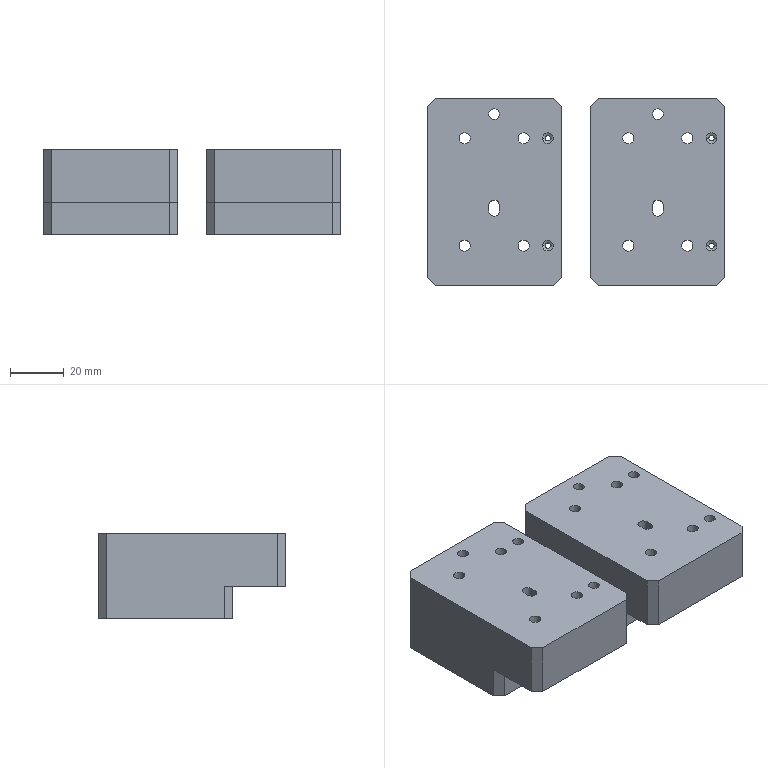NC program | NX | posted with a generic post | part box 111 x 70 x 32 mm
Whole program:
N10 G17 G21 G94 G90
(FLOOR_WALL_COPY , TOOL : D80)
N12 T19 M6
N14 G54
N16 G17 G0 G90 X-43. Y35. S6500 M3
N18 G43 Z30. H19
N20 Z5.
N22 G94 G1 Z2. F1500.
N24 X-40.
N26 X151.
N28 X154.
N30 Z5.
N32 G0 Z30.
N34 X-43.
N36 Z4.
N38 G1 Z1.
N40 X-40.
N42 X151.
N44 X154.
N46 Z4.
N48 G0 Z30.
N50 X-43.
N52 Z3.
N54 G1 Z0.
N56 X-40.
N58 X151.
N60 X154.
N62 Z3.
N64 G0 Z30.
N66 M5
(FLOOR_WALL_1 , TOOL : D10)
N68 T15 M6
N70 G54
N72 G17 G0 G90 X26.443 Y-6.5 S9500 M3
N74 G43 Z30. H15
N76 Z0.508
N78 G94 G1 Z-0.992 F1000.
N80 X25.866 Y-5.5
N82 G3 X25. Y-5. R1.
N84 G1 X0.929 F3500.
N86 X-5. Y0.929
N88 Y20.788
N90 X0.888 Y14.9
N92 X49.112
N94 X55. Y20.788
N96 Y0.929
N98 X49.071 Y-5.
N100 X25.
N102 Y0.
N104 X3.
N106 X0. Y3.
N108 Y9.979
N110 G3 X0.888 Y9.9 R5.
N112 G1 X49.112
N114 G3 X50. Y9.979 R5.
N116 G1 Y3.
N118 X47. Y0.
N120 X25.
N122 Y4.5
N124 X4.864
N126 X4.5 Y4.864
N128 Y5.4
N130 X45.5
N132 Y4.864
N134 X45.136 Y4.5
N136 X25.
N138 G3 X24.134 Y4. R1.
N140 G1 Z0.508
N142 G0 X26.443 Y-6.5 Z-0.483
N144 G1 Z-1.983 F1000.
N146 X25.866 Y-5.5
N148 G3 X25. Y-5. R1.
N150 G1 X0.929 F3500.
N152 X-5. Y0.929
N154 Y20.788
N156 X0.888 Y14.9
N158 X49.112
N160 X55. Y20.788
N162 Y0.929
N164 X49.071 Y-5.
N166 X25.
N168 Y0.
N170 X3.
N172 X0. Y3.
N174 Y9.979
N176 G3 X0.888 Y9.9 R5.
N178 G1 X49.112
N180 G3 X50. Y9.979 R5.
N182 G1 Y3.
N184 X47. Y0.
N186 X25.
N188 Y4.5
N190 X4.864
N192 X4.5 Y4.864
N194 Y5.4
N196 X45.5
N198 Y4.864
N200 X45.136 Y4.5
N202 X25.
N204 G3 X24.134 Y4. R1.
N206 G1 Z-0.483
N208 G0 X26.443 Y-6.5 Z-1.475
N210 G1 Z-2.975 F1000.
N212 X25.866 Y-5.5
N214 G3 X25. Y-5. R1.
N216 G1 X0.929 F3500.
N218 X-5. Y0.929
N220 Y20.788
N222 X0.888 Y14.9
N224 X49.112
N226 X55. Y20.788
N228 Y0.929
N230 X49.071 Y-5.
N232 X25.
N234 Y0.
N236 X3.
N238 X0. Y3.
N240 Y9.979
N242 G3 X0.888 Y9.9 R5.
N244 G1 X49.112
N246 G3 X50. Y9.979 R5.
N248 G1 Y3.
N250 X47. Y0.
N252 X25.
N254 Y4.5
N256 X4.864
N258 X4.5 Y4.864
N260 Y5.4
N262 X45.5
N264 Y4.864
N266 X45.136 Y4.5
N268 X25.
N270 G3 X24.134 Y4. R1.
N272 G1 Z-1.475
N274 G0 X26.443 Y-6.5 Z-2.467
N276 G1 Z-3.967 F1000.
N278 X25.866 Y-5.5
N280 G3 X25. Y-5. R1.
N282 G1 X0.929 F3500.
N284 X-5. Y0.929
N286 Y20.788
N288 X0.888 Y14.9
N290 X49.112
N292 X55. Y20.788
N294 Y0.929
N296 X49.071 Y-5.
N298 X25.
N300 Y0.
N302 X3.
N304 X0. Y3.
N306 Y9.979
N308 G3 X0.888 Y9.9 R5.
N310 G1 X49.112
N312 G3 X50. Y9.979 R5.
N314 G1 Y3.
N316 X47. Y0.
N318 X25.
N320 Y4.5
N322 X4.864
N324 X4.5 Y4.864
N326 Y5.4
N328 X45.5
N330 Y4.864
N332 X45.136 Y4.5
N334 X25.
N336 G3 X24.134 Y4. R1.
N338 G1 Z-2.467
N340 G0 X26.443 Y-6.5 Z-3.458
N342 G1 Z-4.958 F1000.
N344 X25.866 Y-5.5
N346 G3 X25. Y-5. R1.
N348 G1 X0.929 F3500.
N350 X-5. Y0.929
N352 Y20.788
N354 X0.888 Y14.9
N356 X49.112
N358 X55. Y20.788
N360 Y0.929
N362 X49.071 Y-5.
N364 X25.
N366 Y0.
N368 X3.
N370 X0. Y3.
N372 Y9.979
N374 G3 X0.888 Y9.9 R5.
N376 G1 X49.112
N378 G3 X50. Y9.979 R5.
N380 G1 Y3.
N382 X47. Y0.
N384 X25.
N386 Y4.5
N388 X4.864
N390 X4.5 Y4.864
N392 Y5.4
N394 X45.5
N396 Y4.864
N398 X45.136 Y4.5
N400 X25.
N402 G3 X24.134 Y4. R1.
N404 G1 Z-3.458
N406 G0 X26.443 Y-6.5 Z-4.45
N408 G1 Z-5.95 F1000.
N410 X25.866 Y-5.5
N412 G3 X25. Y-5. R1.
N414 G1 X0.929 F3500.
N416 X-5. Y0.929
N418 Y20.788
N420 X0.888 Y14.9
N422 X49.112
N424 X55. Y20.788
N426 Y0.929
N428 X49.071 Y-5.
N430 X25.
N432 Y0.
N434 X3.
N436 X0. Y3.
N438 Y9.979
N440 G3 X0.888 Y9.9 R5.
N442 G1 X49.112
N444 G3 X50. Y9.979 R5.
N446 G1 Y3.
N448 X47. Y0.
N450 X25.
N452 Y4.5
N454 X4.864
N456 X4.5 Y4.864
N458 Y5.4
N460 X45.5
N462 Y4.864
N464 X45.136 Y4.5
N466 X25.
N468 G3 X24.134 Y4. R1.
N470 G1 Z-4.45
N472 G0 X26.443 Y-6.5 Z-5.442
N474 G1 Z-6.942 F1000.
N476 X25.866 Y-5.5
N478 G3 X25. Y-5. R1.
N480 G1 X0.929 F3500.
N482 X-5. Y0.929
N484 Y20.788
N486 X0.888 Y14.9
N488 X49.112
N490 X55. Y20.788
N492 Y0.929
N494 X49.071 Y-5.
N496 X25.
N498 Y0.
N500 X3.
N502 X0. Y3.
N504 Y9.979
N506 G3 X0.888 Y9.9 R5.
N508 G1 X49.112
N510 G3 X50. Y9.979 R5.
N512 G1 Y3.
N514 X47. Y0.
N516 X25.
N518 Y4.5
N520 X4.864
N522 X4.5 Y4.864
N524 Y5.4
N526 X45.5
N528 Y4.864
N530 X45.136 Y4.5
N532 X25.
N534 G3 X24.134 Y4. R1.
N536 G1 Z-5.442
N538 G0 X26.443 Y-6.5 Z-6.433
N540 G1 Z-7.933 F1000.
N542 X25.866 Y-5.5
N544 G3 X25. Y-5. R1.
N546 G1 X0.929 F3500.
N548 X-5. Y0.929
N550 Y20.788
N552 X0.888 Y14.9
N554 X49.112
N556 X55. Y20.788
N558 Y0.929
N560 X49.071 Y-5.
N562 X25.
N564 Y0.
N566 X3.
N568 X0. Y3.
N570 Y9.979
N572 G3 X0.888 Y9.9 R5.
N574 G1 X49.112
N576 G3 X50. Y9.979 R5.
N578 G1 Y3.
N580 X47. Y0.
N582 X25.
N584 Y4.5
N586 X4.864
N588 X4.5 Y4.864
N590 Y5.4
N592 X45.5
N594 Y4.864
N596 X45.136 Y4.5
N598 X25.
N600 G3 X24.134 Y4. R1.
N602 G1 Z-6.433
N604 G0 X26.443 Y-6.5 Z-7.425
N606 G1 Z-8.925 F1000.
N608 X25.866 Y-5.5
N610 G3 X25. Y-5. R1.
N612 G1 X0.929 F3500.
N614 X-5. Y0.929
N616 Y20.788
N618 X0.888 Y14.9
N620 X49.112
N622 X55. Y20.788
N624 Y0.929
N626 X49.071 Y-5.
N628 X25.
N630 Y0.
N632 X3.
N634 X0. Y3.
N636 Y9.979
N638 G3 X0.888 Y9.9 R5.
N640 G1 X49.112
N642 G3 X50. Y9.979 R5.
N644 G1 Y3.
N646 X47. Y0.
N648 X25.
N650 Y4.5
N652 X4.864
N654 X4.5 Y4.864
N656 Y5.4
N658 X45.5
N660 Y4.864
N662 X45.136 Y4.5
N664 X25.
N666 G3 X24.134 Y4. R1.
N668 G1 Z-7.425
N670 G0 X26.443 Y-6.5 Z-8.417
N672 G1 Z-9.917 F1000.
N674 X25.866 Y-5.5
N676 G3 X25. Y-5. R1.
N678 G1 X0.929 F3500.
N680 X-5. Y0.929
N682 Y20.788
N684 X0.888 Y14.9
N686 X49.112
N688 X55. Y20.788
N690 Y0.929
N692 X49.071 Y-5.
N694 X25.
N696 Y0.
N698 X3.
N700 X0. Y3.
N702 Y9.979
N704 G3 X0.888 Y9.9 R5.
N706 G1 X49.112
N708 G3 X50. Y9.979 R5.
N710 G1 Y3.
N712 X47. Y0.
N714 X25.
N716 Y4.5
N718 X4.864
N720 X4.5 Y4.864
N722 Y5.4
N724 X45.5
N726 Y4.864
N728 X45.136 Y4.5
N730 X25.
N732 G3 X24.134 Y4. R1.
N734 G1 Z-8.417
N736 G0 X26.443 Y-6.5 Z-9.408
N738 G1 Z-10.908 F1000.
N740 X25.866 Y-5.5
N742 G3 X25. Y-5. R1.
N744 G1 X0.929 F3500.
N746 X-5. Y0.929
N748 Y20.788
N750 X0.888 Y14.9
N752 X49.112
N754 X55. Y20.788
N756 Y0.929
N758 X49.071 Y-5.
N760 X25.
N762 Y0.
N764 X3.
N766 X0. Y3.
N768 Y9.979
N770 G3 X0.888 Y9.9 R5.
N772 G1 X49.112
N774 G3 X50. Y9.979 R5.
N776 G1 Y3.
N778 X47. Y0.
N780 X25.
N782 Y4.5
N784 X4.864
N786 X4.5 Y4.864
N788 Y5.4
N790 X45.5
N792 Y4.864
N794 X45.136 Y4.5
N796 X25.
N798 G3 X24.134 Y4. R1.
N800 G1 Z-9.408
N802 G0 X26.443 Y-6.5 Z-10.4
N804 G1 Z-11.9 F1000.
N806 X25.866 Y-5.5
N808 G3 X25. Y-5. R1.
N810 G1 X0.929 F3500.
N812 X-5. Y0.929
N814 Y20.788
N816 X0.888 Y14.9
N818 X49.112
N820 X55. Y20.788
N822 Y0.929
N824 X49.071 Y-5.
N826 X25.
N828 Y0.
N830 X3.
N832 X0. Y3.
N834 Y9.979
N836 G3 X0.888 Y9.9 R5.
N838 G1 X49.112
N840 G3 X50. Y9.979 R5.
N842 G1 Y3.
N844 X47. Y0.
N846 X25.
N848 Y4.5
N850 X4.864
N852 X4.5 Y4.864
N854 Y5.4
N856 X45.5
N858 Y4.864
N860 X45.136 Y4.5
N862 X25.
N864 G3 X24.134 Y4. R1.
N866 G1 Z-10.4
N868 G0 Z30.
N870 X87.443 Y-6.5
N872 Z0.508
N874 G1 Z-0.992 F1000.
N876 X86.866 Y-5.5
N878 G3 X86. Y-5. R1.
N880 G1 X61.929 F3500.
N882 X56. Y0.929
N884 Y20.788
N886 X61.888 Y14.9
N888 X110.112
N890 X116. Y20.788
N892 Y0.929
N894 X110.071 Y-5.
N896 X86.
N898 Y0.
N900 X64.
N902 X61. Y3.
N904 Y9.979
N906 G3 X61.888 Y9.9 R5.
N908 G1 X110.112
N910 G3 X111. Y9.979 R5.
N912 G1 Y3.
N914 X108. Y0.
N916 X86.
N918 Y4.5
N920 X65.864
N922 X65.5 Y4.864
N924 Y5.4
N926 X106.5
N928 Y4.864
N930 X106.136 Y4.5
N932 X86.
N934 G3 X85.134 Y4. R1.
N936 G1 Z0.508
N938 G0 X87.443 Y-6.5 Z-0.483
N940 G1 Z-1.983 F1000.
N942 X86.866 Y-5.5
N944 G3 X86. Y-5. R1.
N946 G1 X61.929 F3500.
N948 X56. Y0.929
N950 Y20.788
N952 X61.888 Y14.9
N954 X110.112
N956 X116. Y20.788
N958 Y0.929
N960 X110.071 Y-5.
N962 X86.
N964 Y0.
N966 X64.
N968 X61. Y3.
N970 Y9.979
N972 G3 X61.888 Y9.9 R5.
N974 G1 X110.112
N976 G3 X111. Y9.979 R5.
N978 G1 Y3.
N980 X108. Y0.
N982 X86.
N984 Y4.5
N986 X65.864
N988 X65.5 Y4.864
N990 Y5.4
N992 X106.5
N994 Y4.864
N996 X106.136 Y4.5
N998 X86.
N1000 G3 X85.134 Y4. R1.
N1002 G1 Z-0.483
N1004 G0 X87.443 Y-6.5 Z-1.475
N1006 G1 Z-2.975 F1000.
N1008 X86.866 Y-5.5
N1010 G3 X86. Y-5. R1.
N1012 G1 X61.929 F3500.
N1014 X56. Y0.929
N1016 Y20.788
N1018 X61.888 Y14.9
N1020 X110.112
N1022 X116. Y20.788
N1024 Y0.929
N1026 X110.071 Y-5.
N1028 X86.
N1030 Y0.
N1032 X64.
N1034 X61. Y3.
N1036 Y9.979
N1038 G3 X61.888 Y9.9 R5.
N1040 G1 X110.112
N1042 G3 X111. Y9.979 R5.
N1044 G1 Y3.
N1046 X108. Y0.
N1048 X86.
N1050 Y4.5
N1052 X65.864
N1054 X65.5 Y4.864
N1056 Y5.4
N1058 X106.5
N1060 Y4.864
N1062 X106.136 Y4.5
N1064 X86.
N1066 G3 X85.134 Y4. R1.
N1068 G1 Z-1.475
N1070 G0 X87.443 Y-6.5 Z-2.467
N1072 G1 Z-3.967 F1000.
N1074 X86.866 Y-5.5
N1076 G3 X86. Y-5. R1.
N1078 G1 X61.929 F3500.
N1080 X56. Y0.929
N1082 Y20.788
N1084 X61.888 Y14.9
N1086 X110.112
N1088 X116. Y20.788
N1090 Y0.929
N1092 X110.071 Y-5.
N1094 X86.
N1096 Y0.
N1098 X64.
N1100 X61. Y3.
N1102 Y9.979
N1104 G3 X61.888 Y9.9 R5.
N1106 G1 X110.112
N1108 G3 X111. Y9.979 R5.
N1110 G1 Y3.
N1112 X108. Y0.
N1114 X86.
N1116 Y4.5
N1118 X65.864
N1120 X65.5 Y4.864
N1122 Y5.4
N1124 X106.5
N1126 Y4.864
N1128 X106.136 Y4.5
N1130 X86.
N1132 G3 X85.134 Y4. R1.
N1134 G1 Z-2.467
N1136 G0 X87.443 Y-6.5 Z-3.458
N1138 G1 Z-4.958 F1000.
N1140 X86.866 Y-5.5
N1142 G3 X86. Y-5. R1.
N1144 G1 X61.929 F3500.
N1146 X56. Y0.929
N1148 Y20.788
N1150 X61.888 Y14.9
N1152 X110.112
N1154 X116. Y20.788
N1156 Y0.929
N1158 X110.071 Y-5.
N1160 X86.
N1162 Y0.
N1164 X64.
N1166 X61. Y3.
N1168 Y9.979
N1170 G3 X61.888 Y9.9 R5.
N1172 G1 X110.112
N1174 G3 X111. Y9.979 R5.
N1176 G1 Y3.
N1178 X108. Y0.
N1180 X86.
N1182 Y4.5
N1184 X65.864
N1186 X65.5 Y4.864
N1188 Y5.4
N1190 X106.5
N1192 Y4.864
N1194 X106.136 Y4.5
N1196 X86.
N1198 G3 X85.134 Y4. R1.
N1200 G1 Z-3.458
N1202 G0 X87.443 Y-6.5 Z-4.45
N1204 G1 Z-5.95 F1000.
N1206 X86.866 Y-5.5
N1208 G3 X86. Y-5. R1.
N1210 G1 X61.929 F3500.
N1212 X56. Y0.929
N1214 Y20.788
N1216 X61.888 Y14.9
N1218 X110.112
N1220 X116. Y20.788
N1222 Y0.929
N1224 X110.071 Y-5.
N1226 X86.
N1228 Y0.
N1230 X64.
N1232 X61. Y3.
N1234 Y9.979
N1236 G3 X61.888 Y9.9 R5.
N1238 G1 X110.112
N1240 G3 X111. Y9.979 R5.
N1242 G1 Y3.
N1244 X108. Y0.
N1246 X86.
N1248 Y4.5
N1250 X65.864
N1252 X65.5 Y4.864
N1254 Y5.4
N1256 X106.5
N1258 Y4.864
N1260 X106.136 Y4.5
N1262 X86.
N1264 G3 X85.134 Y4. R1.
N1266 G1 Z-4.45
N1268 G0 X87.443 Y-6.5 Z-5.442
N1270 G1 Z-6.942 F1000.
N1272 X86.866 Y-5.5
N1274 G3 X86. Y-5. R1.
N1276 G1 X61.929 F3500.
N1278 X56. Y0.929
N1280 Y20.788
N1282 X61.888 Y14.9
N1284 X110.112
N1286 X116. Y20.788
N1288 Y0.929
N1290 X110.071 Y-5.
N1292 X86.
N1294 Y0.
N1296 X64.
N1298 X61. Y3.
N1300 Y9.979
N1302 G3 X61.888 Y9.9 R5.
N1304 G1 X110.112
N1306 G3 X111. Y9.979 R5.
N1308 G1 Y3.
N1310 X108. Y0.
N1312 X86.
N1314 Y4.5
N1316 X65.864
N1318 X65.5 Y4.864
N1320 Y5.4
N1322 X106.5
N1324 Y4.864
N1326 X106.136 Y4.5
N1328 X86.
N1330 G3 X85.134 Y4. R1.
N1332 G1 Z-5.442
N1334 G0 X87.443 Y-6.5 Z-6.433
N1336 G1 Z-7.933 F1000.
N1338 X86.866 Y-5.5
N1340 G3 X86. Y-5. R1.
N1342 G1 X61.929 F3500.
N1344 X56. Y0.929
N1346 Y20.788
N1348 X61.888 Y14.9
N1350 X110.112
N1352 X116. Y20.788
N1354 Y0.929
N1356 X110.071 Y-5.
N1358 X86.
N1360 Y0.
N1362 X64.
N1364 X61. Y3.
N1366 Y9.979
N1368 G3 X61.888 Y9.9 R5.
N1370 G1 X110.112
N1372 G3 X111. Y9.979 R5.
N1374 G1 Y3.
N1376 X108. Y0.
N1378 X86.
N1380 Y4.5
N1382 X65.864
N1384 X65.5 Y4.864
N1386 Y5.4
N1388 X106.5
N1390 Y4.864
N1392 X106.136 Y4.5
N1394 X86.
N1396 G3 X85.134 Y4. R1.
N1398 G1 Z-6.433
N1400 G0 X87.443 Y-6.5 Z-7.425
N1402 G1 Z-8.925 F1000.
N1404 X86.866 Y-5.5
N1406 G3 X86. Y-5. R1.
N1408 G1 X61.929 F3500.
N1410 X56. Y0.929
N1412 Y20.788
N1414 X61.888 Y14.9
N1416 X110.112
N1418 X116. Y20.788
N1420 Y0.929
N1422 X110.071 Y-5.
N1424 X86.
N1426 Y0.
N1428 X64.
N1430 X61. Y3.
N1432 Y9.979
N1434 G3 X61.888 Y9.9 R5.
N1436 G1 X110.112
N1438 G3 X111. Y9.979 R5.
N1440 G1 Y3.
N1442 X108. Y0.
N1444 X86.
N1446 Y4.5
N1448 X65.864
N1450 X65.5 Y4.864
N1452 Y5.4
N1454 X106.5
N1456 Y4.864
N1458 X106.136 Y4.5
N1460 X86.
N1462 G3 X85.134 Y4. R1.
N1464 G1 Z-7.425
N1466 G0 X87.443 Y-6.5 Z-8.417
N1468 G1 Z-9.917 F1000.
N1470 X86.866 Y-5.5
N1472 G3 X86. Y-5. R1.
N1474 G1 X61.929 F3500.
N1476 X56. Y0.929
N1478 Y20.788
N1480 X61.888 Y14.9
N1482 X110.112
N1484 X116. Y20.788
N1486 Y0.929
N1488 X110.071 Y-5.
N1490 X86.
N1492 Y0.
N1494 X64.
N1496 X61. Y3.
N1498 Y9.979
N1500 G3 X61.888 Y9.9 R5.
N1502 G1 X110.112
N1504 G3 X111. Y9.979 R5.
N1506 G1 Y3.
N1508 X108. Y0.
N1510 X86.
N1512 Y4.5
N1514 X65.864
N1516 X65.5 Y4.864
N1518 Y5.4
N1520 X106.5
N1522 Y4.864
N1524 X106.136 Y4.5
N1526 X86.
N1528 G3 X85.134 Y4. R1.
N1530 G1 Z-8.417
N1532 G0 X87.443 Y-6.5 Z-9.408
N1534 G1 Z-10.908 F1000.
N1536 X86.866 Y-5.5
N1538 G3 X86. Y-5. R1.
N1540 G1 X61.929 F3500.
N1542 X56. Y0.929
N1544 Y20.788
N1546 X61.888 Y14.9
N1548 X110.112
N1550 X116. Y20.788
N1552 Y0.929
N1554 X110.071 Y-5.
N1556 X86.
N1558 Y0.
N1560 X64.
N1562 X61. Y3.
N1564 Y9.979
N1566 G3 X61.888 Y9.9 R5.
N1568 G1 X110.112
N1570 G3 X111. Y9.979 R5.
N1572 G1 Y3.
N1574 X108. Y0.
N1576 X86.
N1578 Y4.5
N1580 X65.864
N1582 X65.5 Y4.864
N1584 Y5.4
N1586 X106.5
N1588 Y4.864
N1590 X106.136 Y4.5
N1592 X86.
N1594 G3 X85.134 Y4. R1.
N1596 G1 Z-9.408
N1598 G0 X87.443 Y-6.5 Z-10.4
N1600 G1 Z-11.9 F1000.
N1602 X86.866 Y-5.5
N1604 G3 X86. Y-5. R1.
N1606 G1 X61.929 F3500.
N1608 X56. Y0.929
N1610 Y20.788
N1612 X61.888 Y14.9
N1614 X110.112
N1616 X116. Y20.788
N1618 Y0.929
N1620 X110.071 Y-5.
N1622 X86.
N1624 Y0.
N1626 X64.
N1628 X61. Y3.
N1630 Y9.979
N1632 G3 X61.888 Y9.9 R5.
N1634 G1 X110.112
N1636 G3 X111. Y9.979 R5.
N1638 G1 Y3.
N1640 X108. Y0.
N1642 X86.
N1644 Y4.5
N1646 X65.864
N1648 X65.5 Y4.864
N1650 Y5.4
N1652 X106.5
N1654 Y4.864
N1656 X106.136 Y4.5
N1658 X86.
N1660 G3 X85.134 Y4. R1.
N1662 G1 Z-10.4
N1664 G0 Z30.
N1666 M5
(FLOOR_WALL_1_COPY , TOOL : D10JING)
N1668 T14 M6
N1670 G54
N1672 G17 G0 G90 X-6.5 Y16.82 S9500 M3
N1674 G43 Z30. H14
N1676 Z-10.5
N1678 G94 G1 Z-12. F1000.
N1680 X-5.866 Y15.722
N1682 G3 X-5. Y15.222 R1.
N1684 G1 X0. F1500.
N1686 X0.575 Y14.646
N1688 G3 X0.929 Y14.5 R0.5
N1690 G1 X49.071
N1692 G3 X49.425 Y14.646 R0.5
N1694 G1 X50. Y15.222
N1696 X55.
N1698 Y11.481
N1700 X-5.
N1702 Y7.741
N1704 X55.
N1706 Y4.
N1708 X-5.
N1710 G2 X-5.866 Y4.5 R1.
N1712 G1 X-6.5 Y5.598
N1714 Z-10.5
N1716 G0 X51.319 Y14.42
N1718 G1 Z-12. F1000.
N1720 X54.933 Y20.679
N1722 G3 X55. Y20.929 R0.5
N1724 G1 X49.071 Y15. F1500.
N1726 X0.929
N1728 X-5. Y20.929
N1730 G3 X-5.966 Y21.188 R1.
N1732 G1 X-6.5 Y21.045
N1734 Z-10.5
N1736 G0 Z30.
N1738 X54.5 Y16.82
N1740 Z-10.5
N1742 G1 Z-12. F1000.
N1744 X55.134 Y15.722
N1746 G3 X56. Y15.222 R1.
N1748 G1 X61. F1500.
N1750 X61.575 Y14.646
N1752 G3 X61.929 Y14.5 R0.5
N1754 G1 X110.071
N1756 G3 X110.425 Y14.646 R0.5
N1758 G1 X111. Y15.222
N1760 X116.
N1762 Y11.481
N1764 X56.
N1766 Y7.741
N1768 X116.
N1770 Y4.
N1772 X56.
N1774 G2 X55.134 Y4.5 R1.
N1776 G1 X54.5 Y5.598
N1778 Z-10.5
N1780 G0 Z30.
N1782 X117.5 Y21.045
N1784 Z-10.5
N1786 G1 Z-12. F1000.
N1788 X116.966 Y21.188
N1790 G3 X116. Y20.929 R1.
N1792 G1 X110.071 Y15. F1500.
N1794 X61.929
N1796 X56. Y20.929
N1798 G3 X55.034 Y21.188 R1.
N1800 G1 X54.5 Y18.308
N1802 Z-10.5
N1804 G0 Z30.
N1806 M5
(PLANAR_MILL_COPY_COPY , TOOL : D6A45)
N1808 T01 M6
N1810 G54
N1812 G17 G0 G90 X38.567 Y28.5 S9500 M3
N1814 G43 Z30. H1
N1816 Z0.5
N1818 G94 G1 Z-1. F1250.
N1820 G3 X39. Y28.25 R0.5
N1822 X39.75 Y29. R0.75
N1824 X39. Y28.25 R-0.75
N1826 X39.433 Y28.5 R0.5
N1828 G1 Z0.5
N1830 G0 Z30.
N1832 X10.567
N1834 Z0.5
N1836 G1 Z-1.
N1838 G3 X11. Y28.25 R0.5
N1840 X11.75 Y29. R0.75
N1842 X11. Y28.25 R-0.75
N1844 X11.433 Y28.5 R0.5
N1846 G1 Z0.5
N1848 G0 Z30.
N1850 X5.085 Y55.098
N1852 Z0.5
N1854 G1 X4.9 Y55.083 Z0.448
N1856 X4.917 Y54.9 Z0.397
N1858 X5.1 Y54.917 Z0.346
N1860 X5.083 Y55.1 Z0.296
N1862 X4.9 Y55.083 Z0.245
N1864 X4.917 Y54.9 Z0.194
N1866 X5.1 Y54.917 Z0.143
N1868 X5.083 Y55.1 Z0.092
N1870 X4.9 Y55.083 Z0.041
N1872 X4.917 Y54.9 Z-0.01
N1874 X5.1 Y54.917 Z-0.061
N1876 X5.083 Y55.1 Z-0.112
N1878 X4.9 Y55.083 Z-0.163
N1880 X4.917 Y54.9 Z-0.214
N1882 X5.1 Y54.917 Z-0.265
N1884 X5.083 Y55.1 Z-0.316
N1886 X4.9 Y55.083 Z-0.367
N1888 X4.917 Y54.9 Z-0.417
N1890 X5.1 Y54.917 Z-0.468
N1892 X5.083 Y55.1 Z-0.519
N1894 X4.9 Y55.083 Z-0.57
N1896 X4.917 Y54.9 Z-0.621
N1898 X5.1 Y54.917 Z-0.672
N1900 X5.083 Y55.1 Z-0.723
N1902 X4.9 Y55.083 Z-0.774
N1904 X4.917 Y54.9 Z-0.825
N1906 X5.1 Y54.917 Z-0.876
N1908 X5.083 Y55.1 Z-0.927
N1910 X4.9 Y55.083 Z-0.978
N1912 Y55. Z-1.
N1914 G3 X5. Y54.9 R0.1
N1916 X4.9 Y55. R-0.1
N1918 G1 Z0.5
N1920 G0 Z30.
N1922 X11.433 Y64.5
N1924 Z0.5
N1926 G1 Z-1.
N1928 G3 X11. Y64.75 R0.5
N1930 X10.25 Y64. R0.75
N1932 X11. Y64.75 R-0.75
N1934 X10.567 Y64.5 R0.5
N1936 G1 Z0.5
N1938 G0 Z30.
N1940 X13.3 Y55.866
N1942 Z0.5
N1944 G1 Z-1.
N1946 G3 X12.8 Y55. R1.
N1948 X14. Y53.8 R1.2
N1950 X12.8 Y55. R-1.2
N1952 X13.3 Y54.134 R1.
N1954 G1 Z0.5
N1956 G0 Z30.
N1958 X-1.4 Y44.134
N1960 Z0.5
N1962 G1 Z-1.
N1964 G3 X-0.9 Y45. R1.
N1966 G1 Y67.
N1968 G2 X-0.636 Y67.636 R0.9
N1970 G1 X2.364 Y70.636
N1972 G2 X3. Y70.9 R0.9
N1974 G1 X47.
N1976 G2 X47.636 Y70.636 R0.9
N1978 G1 X50.636 Y67.636
N1980 G2 X50.9 Y67. R0.9
N1982 G1 Y23.
N1984 G2 X50.636 Y22.364 R0.9
N1986 G1 X47.636 Y19.364
N1988 G2 X47. Y19.1 R0.9
N1990 G1 X3.
N1992 G2 X2.364 Y19.364 R0.9
N1994 G1 X-0.636 Y22.364
N1996 G2 X-0.9 Y23. R0.9
N1998 G1 Y45.
N2000 G3 X-1.4 Y45.866 R1.
N2002 G1 Z0.5
N2004 G0 Z30.
N2006 X36.866 Y55.7
N2008 Z0.5
N2010 G1 Z-1.
N2012 G3 X36. Y56.2 R1.
N2014 X34.8 Y55. R1.2
N2016 X36. Y56.2 R-1.2
N2018 X35.134 Y55.7 R1.
N2020 G1 Z0.5
N2022 G0 Z30.
N2024 X39.433 Y64.5
N2026 Z0.5
N2028 G1 Z-1.
N2030 G3 X39. Y64.75 R0.5
N2032 X38.25 Y64. R0.75
N2034 X39. Y64.75 R-0.75
N2036 X38.567 Y64.5 R0.5
N2038 G1 Z0.5
N2040 G0 Z30.
N2042 X66.098 Y54.915
N2044 Z0.5
N2046 G1 X66.083 Y55.1 Z0.448
N2048 X65.9 Y55.083 Z0.397
N2050 X65.917 Y54.9 Z0.346
N2052 X66.1 Y54.917 Z0.296
N2054 X66.083 Y55.1 Z0.245
N2056 X65.9 Y55.083 Z0.194
N2058 X65.917 Y54.9 Z0.143
N2060 X66.1 Y54.917 Z0.092
N2062 X66.083 Y55.1 Z0.041
N2064 X65.9 Y55.083 Z-0.01
N2066 X65.917 Y54.9 Z-0.061
N2068 X66.1 Y54.917 Z-0.112
N2070 X66.083 Y55.1 Z-0.163
N2072 X65.9 Y55.083 Z-0.214
N2074 X65.917 Y54.9 Z-0.265
N2076 X66.1 Y54.917 Z-0.316
N2078 X66.083 Y55.1 Z-0.367
N2080 X65.9 Y55.083 Z-0.417
N2082 X65.917 Y54.9 Z-0.468
N2084 X66.1 Y54.917 Z-0.519
N2086 X66.083 Y55.1 Z-0.57
N2088 X65.9 Y55.083 Z-0.621
N2090 X65.917 Y54.9 Z-0.672
N2092 X66.1 Y54.917 Z-0.723
N2094 X66.083 Y55.1 Z-0.774
N2096 X65.9 Y55.083 Z-0.825
N2098 X65.917 Y54.9 Z-0.876
N2100 X66.1 Y54.917 Z-0.927
N2102 X66.083 Y55.1 Z-0.978
N2104 X66. Z-1.
N2106 G3 X65.9 Y55. R0.1
N2108 X66. Y55.1 R-0.1
N2110 G1 Z0.5
N2112 G0 Z30.
N2114 X72.433 Y64.5
N2116 Z0.5
N2118 G1 Z-1.
N2120 G3 X72. Y64.75 R0.5
N2122 X71.25 Y64. R0.75
N2124 X72. Y64.75 R-0.75
N2126 X71.567 Y64.5 R0.5
N2128 G1 Z0.5
N2130 G0 Z30.
N2132 X75.866 Y55.7
N2134 Z0.5
N2136 G1 Z-1.
N2138 G3 X75. Y56.2 R1.
N2140 X73.8 Y55. R1.2
N2142 X75. Y56.2 R-1.2
N2144 X74.134 Y55.7 R1.
N2146 G1 Z0.5
N2148 G0 Z30.
N2150 X85.134 Y71.4
N2152 Z0.5
N2154 G1 Z-1.
N2156 G3 X86. Y70.9 R1.
N2158 G1 X108.
N2160 G2 X108.636 Y70.636 R0.9
N2162 G1 X111.636 Y67.636
N2164 G2 X111.9 Y67. R0.9
N2166 G1 Y23.
N2168 G2 X111.636 Y22.364 R0.9
N2170 G1 X108.636 Y19.364
N2172 G2 X108. Y19.1 R0.9
N2174 G1 X64.
N2176 G2 X63.364 Y19.364 R0.9
N2178 G1 X60.364 Y22.364
N2180 G2 X60.1 Y23. R0.9
N2182 G1 Y67.
N2184 G2 X60.364 Y67.636 R0.9
N2186 G1 X63.364 Y70.636
N2188 G2 X64. Y70.9 R0.9
N2190 G1 X86.
N2192 G3 X86.866 Y71.4 R1.
N2194 G1 Z0.5
N2196 G0 Z30.
N2198 X71.567 Y28.5
N2200 Z0.5
N2202 G1 Z-1.
N2204 G3 X72. Y28.25 R0.5
N2206 X72.75 Y29. R0.75
N2208 X72. Y28.25 R-0.75
N2210 X72.433 Y28.5 R0.5
N2212 G1 Z0.5
N2214 G0 Z30.
N2216 X99.567
N2218 Z0.5
N2220 G1 Z-1.
N2222 G3 X100. Y28.25 R0.5
N2224 X100.75 Y29. R0.75
N2226 X100. Y28.25 R-0.75
N2228 X100.433 Y28.5 R0.5
N2230 G1 Z0.5
N2232 G0 Z30.
N2234 X97.7 Y54.134
N2236 Z0.5
N2238 G1 Z-1.
N2240 G3 X98.2 Y55. R1.
N2242 X97. Y56.2 R1.2
N2244 X98.2 Y55. R-1.2
N2246 X97.7 Y55.866 R1.
N2248 G1 Z0.5
N2250 G0 Z30.
N2252 X100.433 Y64.5
N2254 Z0.5
N2256 G1 Z-1.
N2258 G3 X100. Y64.75 R0.5
N2260 X99.25 Y64. R0.75
N2262 X100. Y64.75 R-0.75
N2264 X99.567 Y64.5 R0.5
N2266 G1 Z0.5
N2268 G0 Z30.
(PLANAR_MILL_COPY_COPY_COPY , TOOL : D6A45)
N2270 X96.87 Y16.2
N2272 Z-11.5
N2274 G1 X96.73 Z-11.538
N2276 X96.13 Y15.87 Z-11.721
N2278 X95.8 Y15.27 Z-11.904
N2280 Y14.73 Z-12.049
N2282 X96.13 Y14.13 Z-12.233
N2284 X96.73 Y13.8 Z-12.416
N2286 X97.27 Z-12.561
N2288 X97.87 Y14.13 Z-12.744
N2290 X98.2 Y14.73 Z-12.928
N2292 Y15. Z-13.
N2294 G3 X97. Y16.2 R1.2
N2296 X98.2 Y15. R-1.2
N2298 X97.7 Y15.866 R1.
N2300 G1 Z-11.5
N2302 G0 Z30.
N2304 X76.2 Y15.13
N2306 Z-11.5
N2308 G1 Y15.27 Z-11.538
N2310 X75.87 Y15.87 Z-11.721
N2312 X75.27 Y16.2 Z-11.904
N2314 X74.73 Z-12.049
N2316 X74.13 Y15.87 Z-12.233
N2318 X73.8 Y15.27 Z-12.416
N2320 Y14.73 Z-12.561
N2322 X74.13 Y14.13 Z-12.744
N2324 X74.73 Y13.8 Z-12.928
N2326 X75. Z-13.
N2328 G3 X76.2 Y15. R1.2
N2330 X75. Y13.8 R-1.2
N2332 X75.866 Y14.3 R1.
N2334 G1 Z-11.5
N2336 G0 Z30.
N2338 X65.902 Y15.085
N2340 Z-11.5
N2342 G1 X65.917 Y14.9 Z-11.552
N2344 X66.1 Y14.917 Z-11.603
N2346 X66.083 Y15.1 Z-11.654
N2348 X65.9 Y15.083 Z-11.704
N2350 X65.917 Y14.9 Z-11.755
N2352 X66.1 Y14.917 Z-11.806
N2354 X66.083 Y15.1 Z-11.857
N2356 X65.9 Y15.083 Z-11.908
N2358 X65.917 Y14.9 Z-11.959
N2360 X66.1 Y14.917 Z-12.01
N2362 X66.083 Y15.1 Z-12.061
N2364 X65.9 Y15.083 Z-12.112
N2366 X65.917 Y14.9 Z-12.163
N2368 X66.1 Y14.917 Z-12.214
N2370 X66.083 Y15.1 Z-12.265
N2372 X65.9 Y15.083 Z-12.316
N2374 X65.917 Y14.9 Z-12.367
N2376 X66.1 Y14.917 Z-12.417
N2378 X66.083 Y15.1 Z-12.468
N2380 X65.9 Y15.083 Z-12.519
N2382 X65.917 Y14.9 Z-12.57
N2384 X66.1 Y14.917 Z-12.621
N2386 X66.083 Y15.1 Z-12.672
N2388 X65.9 Y15.083 Z-12.723
N2390 X65.917 Y14.9 Z-12.774
N2392 X66.1 Y14.917 Z-12.825
N2394 X66.083 Y15.1 Z-12.876
N2396 X65.9 Y15.083 Z-12.927
N2398 X65.917 Y14.9 Z-12.978
N2400 X66. Z-13.
N2402 G3 X66.1 Y15. R0.1
N2404 X66. Y14.9 R-0.1
N2406 G1 Z-11.5
N2408 G0 Z30.
N2410 X52.647 Y19.
N2412 Z-11.5
N2414 G1 Z-13.
N2416 X51.866 Y19.209
N2418 G3 X50.9 Y18.95 R1.
N2420 G1 Y3.041
N2422 G2 X50.607 Y2.334 R1.
N2424 G1 X47.666 Y-0.607
N2426 G2 X46.959 Y-0.9 R1.
N2428 G1 X3.041
N2430 G2 X2.334 Y-0.607 R1.
N2432 G1 X-0.607 Y2.334
N2434 G2 X-0.9 Y3.041 R1.
N2436 G1 Y18.95
N2438 G3 X-1.866 Y19.209 R1.
N2440 G1 X-2.647 Y19.
N2442 Z-11.5
N2444 G0 Z30.
N2446 X113.647
N2448 Z-11.5
N2450 G1 Z-13.
N2452 X112.866 Y19.209
N2454 G3 X111.9 Y18.95 R1.
N2456 G1 Y3.041
N2458 G2 X111.607 Y2.334 R1.
N2460 G1 X108.666 Y-0.607
N2462 G2 X107.959 Y-0.9 R1.
N2464 G1 X64.041
N2466 G2 X63.334 Y-0.607 R1.
N2468 G1 X60.393 Y2.334
N2470 G2 X60.1 Y3.041 R1.
N2472 G1 Y18.95
N2474 G3 X59.134 Y19.209 R1.
N2476 G1 X58.353 Y19.
N2478 Z-11.5
N2480 G0 Z30.
N2482 X37.2 Y15.13
N2484 Z-11.5
N2486 G1 Y15.27 Z-11.538
N2488 X36.87 Y15.87 Z-11.721
N2490 X36.27 Y16.2 Z-11.904
N2492 X35.73 Z-12.049
N2494 X35.13 Y15.87 Z-12.233
N2496 X34.8 Y15.27 Z-12.416
N2498 Y14.73 Z-12.561
N2500 X35.13 Y14.13 Z-12.744
N2502 X35.73 Y13.8 Z-12.928
N2504 X36. Z-13.
N2506 G3 X37.2 Y15. R1.2
N2508 X36. Y13.8 R-1.2
N2510 X36.866 Y14.3 R1.
N2512 G1 Z-11.5
N2514 G0 Z30.
N2516 X14.13 Y13.8
N2518 Z-11.5
N2520 G1 X14.27 Z-11.538
N2522 X14.87 Y14.13 Z-11.721
N2524 X15.2 Y14.73 Z-11.904
N2526 Y15.27 Z-12.049
N2528 X14.87 Y15.87 Z-12.233
N2530 X14.27 Y16.2 Z-12.416
N2532 X13.73 Z-12.561
N2534 X13.13 Y15.87 Z-12.744
N2536 X12.8 Y15.27 Z-12.928
N2538 Y15. Z-13.
N2540 G3 X14. Y13.8 R1.2
N2542 X12.8 Y15. R-1.2
N2544 X13.3 Y14.134 R1.
N2546 G1 Z-11.5
N2548 G0 Z30.
N2550 X5.085 Y15.098
N2552 Z-11.5
N2554 G1 X4.9 Y15.083 Z-11.552
N2556 X4.917 Y14.9 Z-11.603
N2558 X5.1 Y14.917 Z-11.654
N2560 X5.083 Y15.1 Z-11.704
N2562 X4.9 Y15.083 Z-11.755
N2564 X4.917 Y14.9 Z-11.806
N2566 X5.1 Y14.917 Z-11.857
N2568 X5.083 Y15.1 Z-11.908
N2570 X4.9 Y15.083 Z-11.959
N2572 X4.917 Y14.9 Z-12.01
N2574 X5.1 Y14.917 Z-12.061
N2576 X5.083 Y15.1 Z-12.112
N2578 X4.9 Y15.083 Z-12.163
N2580 X4.917 Y14.9 Z-12.214
N2582 X5.1 Y14.917 Z-12.265
N2584 X5.083 Y15.1 Z-12.316
N2586 X4.9 Y15.083 Z-12.367
N2588 X4.917 Y14.9 Z-12.417
N2590 X5.1 Y14.917 Z-12.468
N2592 X5.083 Y15.1 Z-12.519
N2594 X4.9 Y15.083 Z-12.57
N2596 X4.917 Y14.9 Z-12.621
N2598 X5.1 Y14.917 Z-12.672
N2600 X5.083 Y15.1 Z-12.723
N2602 X4.9 Y15.083 Z-12.774
N2604 X4.917 Y14.9 Z-12.825
N2606 X5.1 Y14.917 Z-12.876
N2608 X5.083 Y15.1 Z-12.927
N2610 X4.9 Y15.083 Z-12.978
N2612 Y15. Z-13.
N2614 G3 X5. Y14.9 R0.1
N2616 X4.9 Y15. R-0.1
N2618 G1 Z-11.5
N2620 G0 Z30.
N2622 M5
N2624 M2